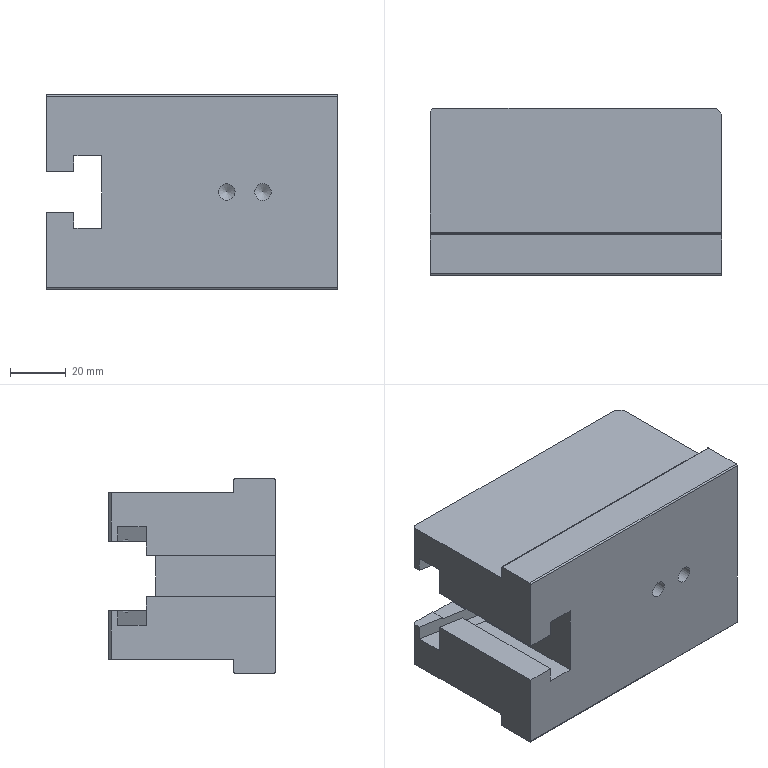Part | STEP file | solid 152 | 1 solid | 48 faces | box 105 x 60 x 70 mm | volume 303902 mm3 | plane 38 | cylinder 8 | cone 2 | commonest cylinder face diameters 1 x6 6 x2